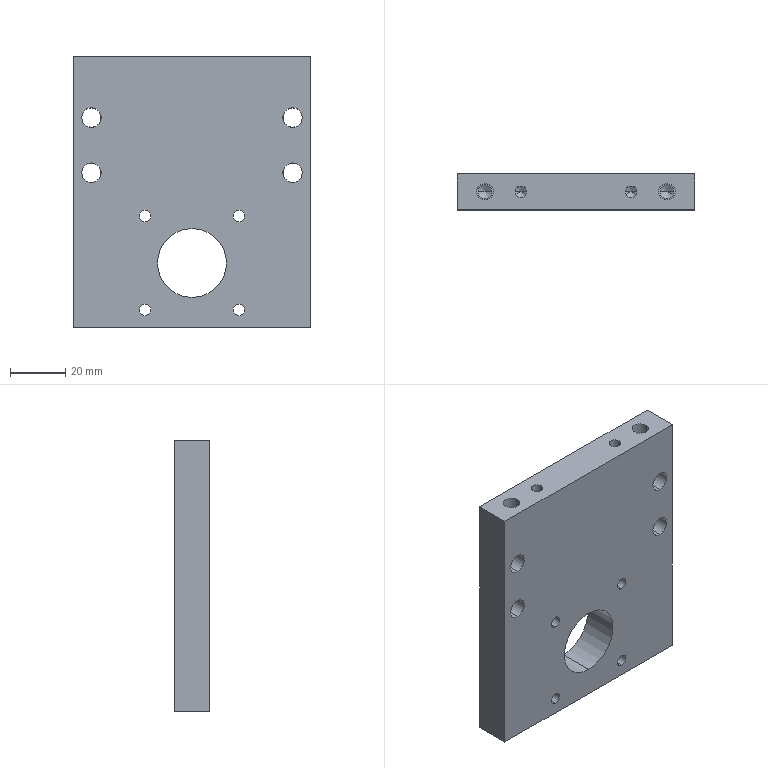Part | STEP file | OP10-121_cylinder stand (2) -R | 1 solid | 74 faces | box 86 x 13 x 98 mm | volume 98029 mm3 | cylinder 38 | cone 24 | plane 12 | commonest cylinder face diameters 4.2 x12 7 x8 11 x8 5 x4 6 x4 25 x2